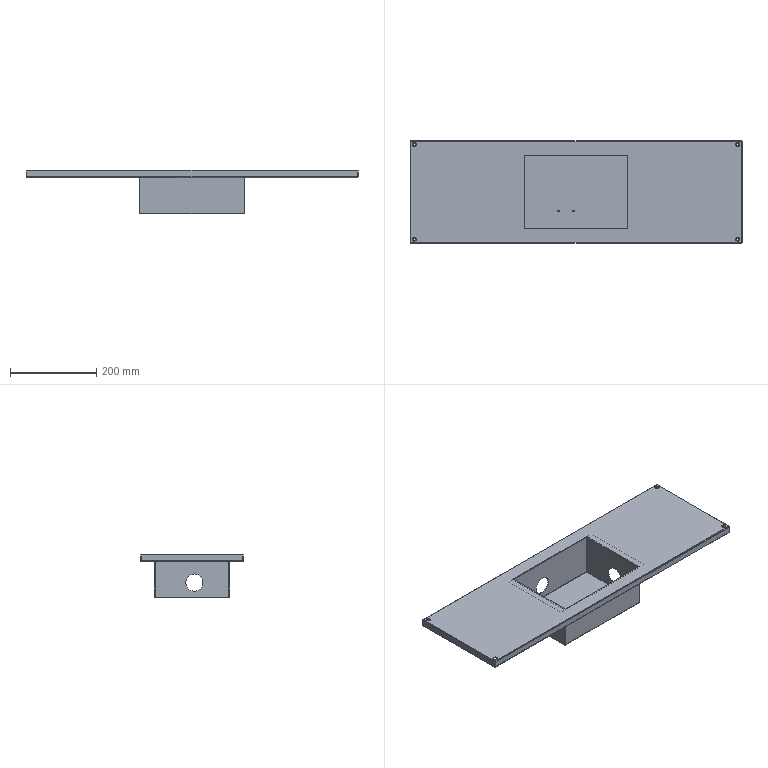Part | SolidWorks | features EdgeFlange 4, Cut 3, FlatPattern 2, HoleWzd 2, SMBaseFlange 2, SheetMetal 2, ICE 1 | 2 solids | 166 faces | box 768 x 238 x 101.5 mm | volume 482103 mm3 | plane 84 | cylinder 58 | spline 24 | commonest cylinder face diameters 1 x14 4 x14 5.8 x12 10 x8 40 x6 4.2 x4